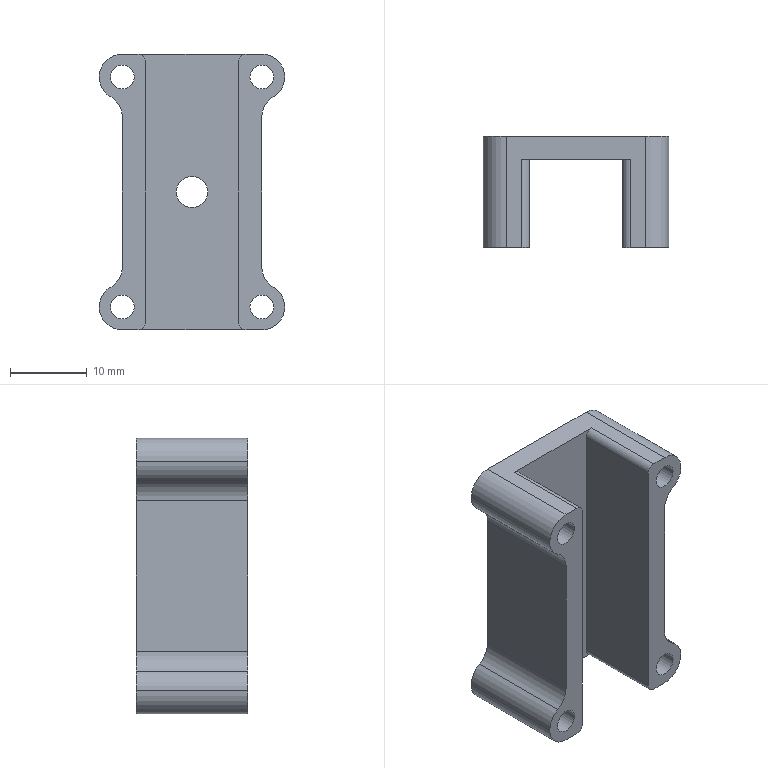Part | SolidWorks | features Fillet 2, ICE 2, Extrusion 1 | 1 solid | 34 faces | box 24.2 x 14.5 x 36 mm | volume 4824 mm3 | cylinder 24 | plane 10 | commonest cylinder face diameters 6 x10 3.1 x8 2 x4 4.1 x2
STEP:
#1=CARTESIAN_POINT('',(2.05,6.,18.));
#2=VERTEX_POINT('',#1);
#3=CARTESIAN_POINT('',(-2.05,6.,18.));
#4=VERTEX_POINT('',#3);
#5=CARTESIAN_POINT('',(0.,6.,18.));
#6=DIRECTION('',(0.,1.,0.));
#7=DIRECTION('',(0.,0.,1.));
#8=AXIS2_PLACEMENT_3D('',#5,#6,#7);
#9=CIRCLE('',#8,2.05);
#10=EDGE_CURVE('',#2,#4,#9,.T.);
#11=ORIENTED_EDGE('',*,*,#10,.F.);
#12=CARTESIAN_POINT('',(2.05,9.,18.));
#13=VERTEX_POINT('',#12);
#14=CARTESIAN_POINT('',(2.05,-5.5,18.));
#15=DIRECTION('',(0.,1.,0.));
#16=VECTOR('',#15,1000.);
#17=LINE('',#14,#16);
#18=EDGE_CURVE('',#2,#13,#17,.T.);
#19=ORIENTED_EDGE('',*,*,#18,.T.);
#20=CARTESIAN_POINT('',(-2.05,9.,18.));
#21=VERTEX_POINT('',#20);
#22=CARTESIAN_POINT('',(0.,9.,18.));
#23=DIRECTION('',(0.,1.,0.));
#24=DIRECTION('',(-1.,0.,0.));
#25=AXIS2_PLACEMENT_3D('',#22,#23,#24);
#26=CIRCLE('',#25,2.05);
#27=EDGE_CURVE('',#13,#21,#26,.T.);
#28=ORIENTED_EDGE('',*,*,#27,.T.);
#29=CARTESIAN_POINT('',(-2.05,-5.5,18.));
#30=DIRECTION('',(0.,1.,0.));
#31=VECTOR('',#30,1000.);
#32=LINE('',#29,#31);
#33=EDGE_CURVE('',#4,#21,#32,.T.);
#34=ORIENTED_EDGE('',*,*,#33,.F.);
#35=EDGE_LOOP('',(#11,#19,#28,#34));
#36=FACE_OUTER_BOUND('',#35,.T.);
#37=CARTESIAN_POINT('',(0.,-5.5,18.));
#38=DIRECTION('',(0.,1.,0.));
#39=DIRECTION('',(-1.,0.,0.));
#40=AXIS2_PLACEMENT_3D('',#37,#38,#39);
#41=CYLINDRICAL_SURFACE('',#40,2.05);
#42=ADVANCED_FACE('',(#36),#41,.F.);
#43=CARTESIAN_POINT('',(10.65,-5.5,33.));
#44=VERTEX_POINT('',#43);
#45=CARTESIAN_POINT('',(7.55,-5.5,33.));
#46=VERTEX_POINT('',#45);
#47=CARTESIAN_POINT('',(9.1,-5.5,33.));
#48=DIRECTION('',(0.,1.,0.));
#49=DIRECTION('',(-1.,0.,0.));
#50=AXIS2_PLACEMENT_3D('',#47,#48,#49);
#51=CIRCLE('',#50,1.55);
#52=EDGE_CURVE('',#44,#46,#51,.T.);
#53=ORIENTED_EDGE('',*,*,#52,.F.);
#54=CARTESIAN_POINT('',(10.65,9.,33.));
#55=VERTEX_POINT('',#54);
#56=CARTESIAN_POINT('',(10.65,-5.5,33.));
#57=DIRECTION('',(0.,1.,0.));
#58=VECTOR('',#57,1000.);
#59=LINE('',#56,#58);
#60=EDGE_CURVE('',#44,#55,#59,.T.);
#61=ORIENTED_EDGE('',*,*,#60,.T.);
#62=CARTESIAN_POINT('',(7.55,9.,33.));
#63=VERTEX_POINT('',#62);
#64=CARTESIAN_POINT('',(9.1,9.,33.));
#65=DIRECTION('',(0.,1.,0.));
#66=DIRECTION('',(-1.,0.,0.));
#67=AXIS2_PLACEMENT_3D('',#64,#65,#66);
#68=CIRCLE('',#67,1.55);
#69=EDGE_CURVE('',#55,#63,#68,.T.);
#70=ORIENTED_EDGE('',*,*,#69,.T.);
#71=CARTESIAN_POINT('',(7.55,-5.5,33.));
#72=DIRECTION('',(0.,1.,0.));
#73=VECTOR('',#72,1000.);
#74=LINE('',#71,#73);
#75=EDGE_CURVE('',#46,#63,#74,.T.);
#76=ORIENTED_EDGE('',*,*,#75,.F.);
#77=EDGE_LOOP('',(#53,#61,#70,#76));
#78=FACE_OUTER_BOUND('',#77,.T.);
#79=CARTESIAN_POINT('',(9.1,-5.5,33.));
#80=DIRECTION('',(0.,1.,0.));
#81=DIRECTION('',(-1.,0.,0.));
#82=AXIS2_PLACEMENT_3D('',#79,#80,#81);
#83=CYLINDRICAL_SURFACE('',#82,1.55);
#84=ADVANCED_FACE('',(#78),#83,.F.);
#85=CARTESIAN_POINT('',(10.65,-5.5,3.));
#86=VERTEX_POINT('',#85);
#87=CARTESIAN_POINT('',(7.55,-5.5,3.));
#88=VERTEX_POINT('',#87);
#89=CARTESIAN_POINT('',(9.1,-5.5,3.));
#90=DIRECTION('',(0.,1.,0.));
#91=DIRECTION('',(-1.,0.,0.));
#92=AXIS2_PLACEMENT_3D('',#89,#90,#91);
#93=CIRCLE('',#92,1.55);
#94=EDGE_CURVE('',#86,#88,#93,.T.);
#95=ORIENTED_EDGE('',*,*,#94,.F.);
#96=CARTESIAN_POINT('',(10.65,9.,3.));
#97=VERTEX_POINT('',#96);
#98=CARTESIAN_POINT('',(10.65,-5.5,3.));
#99=DIRECTION('',(0.,1.,0.));
#100=VECTOR('',#99,1000.);
#101=LINE('',#98,#100);
#102=EDGE_CURVE('',#86,#97,#101,.T.);
#103=ORIENTED_EDGE('',*,*,#102,.T.);
#104=CARTESIAN_POINT('',(7.55,9.,3.));
#105=VERTEX_POINT('',#104);
#106=CARTESIAN_POINT('',(9.1,9.,3.));
#107=DIRECTION('',(0.,1.,0.));
#108=DIRECTION('',(-1.,0.,0.));
#109=AXIS2_PLACEMENT_3D('',#106,#107,#108);
#110=CIRCLE('',#109,1.55);
#111=EDGE_CURVE('',#97,#105,#110,.T.);
#112=ORIENTED_EDGE('',*,*,#111,.T.);
#113=CARTESIAN_POINT('',(7.55,-5.5,3.));
#114=DIRECTION('',(0.,1.,0.));
#115=VECTOR('',#114,1000.);
#116=LINE('',#113,#115);
#117=EDGE_CURVE('',#88,#105,#116,.T.);
#118=ORIENTED_EDGE('',*,*,#117,.F.);
#119=EDGE_LOOP('',(#95,#103,#112,#118));
#120=FACE_OUTER_BOUND('',#119,.T.);
#121=CARTESIAN_POINT('',(9.1,-5.5,3.));
#122=DIRECTION('',(0.,1.,0.));
#123=DIRECTION('',(-1.,0.,0.));
#124=AXIS2_PLACEMENT_3D('',#121,#122,#123);
#125=CYLINDRICAL_SURFACE('',#124,1.55);
#126=ADVANCED_FACE('',(#120),#125,.F.);
#127=CARTESIAN_POINT('',(-7.55,-5.5,3.));
#128=VERTEX_POINT('',#127);
#129=CARTESIAN_POINT('',(-10.65,-5.5,3.));
#130=VERTEX_POINT('',#129);
#131=CARTESIAN_POINT('',(-9.1,-5.5,3.));
#132=DIRECTION('',(0.,1.,0.));
#133=DIRECTION('',(-1.,0.,0.));
#134=AXIS2_PLACEMENT_3D('',#131,#132,#133);
#135=CIRCLE('',#134,1.55);
#136=EDGE_CURVE('',#128,#130,#135,.T.);
#137=ORIENTED_EDGE('',*,*,#136,.F.);
#138=CARTESIAN_POINT('',(-7.55,9.,3.));
#139=VERTEX_POINT('',#138);
#140=CARTESIAN_POINT('',(-7.55,-5.5,3.));
#141=DIRECTION('',(0.,1.,0.));
#142=VECTOR('',#141,1000.);
#143=LINE('',#140,#142);
#144=EDGE_CURVE('',#128,#139,#143,.T.);
#145=ORIENTED_EDGE('',*,*,#144,.T.);
#146=CARTESIAN_POINT('',(-10.65,9.,3.));
#147=VERTEX_POINT('',#146);
#148=CARTESIAN_POINT('',(-9.1,9.,3.));
#149=DIRECTION('',(0.,1.,0.));
#150=DIRECTION('',(-1.,0.,0.));
#151=AXIS2_PLACEMENT_3D('',#148,#149,#150);
#152=CIRCLE('',#151,1.55);
#153=EDGE_CURVE('',#139,#147,#152,.T.);
#154=ORIENTED_EDGE('',*,*,#153,.T.);
#155=CARTESIAN_POINT('',(-10.65,-5.5,3.));
#156=DIRECTION('',(0.,1.,0.));
#157=VECTOR('',#156,1000.);
#158=LINE('',#155,#157);
#159=EDGE_CURVE('',#130,#147,#158,.T.);
#160=ORIENTED_EDGE('',*,*,#159,.F.);
#161=EDGE_LOOP('',(#137,#145,#154,#160));
#162=FACE_OUTER_BOUND('',#161,.T.);
#163=CARTESIAN_POINT('',(-9.1,-5.5,3.));
#164=DIRECTION('',(0.,1.,0.));
#165=DIRECTION('',(-1.,0.,0.));
#166=AXIS2_PLACEMENT_3D('',#163,#164,#165);
#167=CYLINDRICAL_SURFACE('',#166,1.55);
#168=ADVANCED_FACE('',(#162),#167,.F.);
#169=CARTESIAN_POINT('',(-7.55,-5.5,33.));
#170=VERTEX_POINT('',#169);
#171=CARTESIAN_POINT('',(-10.65,-5.5,33.));
#172=VERTEX_POINT('',#171);
#173=CARTESIAN_POINT('',(-9.1,-5.5,33.));
#174=DIRECTION('',(0.,1.,0.));
#175=DIRECTION('',(-1.,0.,0.));
#176=AXIS2_PLACEMENT_3D('',#173,#174,#175);
#177=CIRCLE('',#176,1.55);
#178=EDGE_CURVE('',#170,#172,#177,.T.);
#179=ORIENTED_EDGE('',*,*,#178,.F.);
#180=CARTESIAN_POINT('',(-7.55,9.,33.));
#181=VERTEX_POINT('',#180);
#182=CARTESIAN_POINT('',(-7.55,-5.5,33.));
#183=DIRECTION('',(0.,1.,0.));
#184=VECTOR('',#183,1000.);
#185=LINE('',#182,#184);
#186=EDGE_CURVE('',#170,#181,#185,.T.);
#187=ORIENTED_EDGE('',*,*,#186,.T.);
#188=CARTESIAN_POINT('',(-10.65,9.,33.));
#189=VERTEX_POINT('',#188);
#190=CARTESIAN_POINT('',(-9.1,9.,33.));
#191=DIRECTION('',(0.,1.,0.));
#192=DIRECTION('',(-1.,0.,0.));
#193=AXIS2_PLACEMENT_3D('',#190,#191,#192);
#194=CIRCLE('',#193,1.55);
#195=EDGE_CURVE('',#181,#189,#194,.T.);
#196=ORIENTED_EDGE('',*,*,#195,.T.);
#197=CARTESIAN_POINT('',(-10.65,-5.5,33.));
#198=DIRECTION('',(0.,1.,0.));
#199=VECTOR('',#198,1000.);
#200=LINE('',#197,#199);
#201=EDGE_CURVE('',#172,#189,#200,.T.);
#202=ORIENTED_EDGE('',*,*,#201,.F.);
#203=EDGE_LOOP('',(#179,#187,#196,#202));
#204=FACE_OUTER_BOUND('',#203,.T.);
#205=CARTESIAN_POINT('',(-9.1,-5.5,33.));
#206=DIRECTION('',(0.,1.,0.));
#207=DIRECTION('',(-1.,0.,0.));
#208=AXIS2_PLACEMENT_3D('',#205,#206,#207);
#209=CYLINDRICAL_SURFACE('',#208,1.55);
#210=ADVANCED_FACE('',(#204),#209,.F.);
#211=CARTESIAN_POINT('',(-12.1,-5.5,33.));
#212=VERTEX_POINT('',#211);
#213=CARTESIAN_POINT('',(-10.6,-5.5,30.402));
#214=VERTEX_POINT('',#213);
#215=CARTESIAN_POINT('',(-9.1,-5.5,33.));
#216=DIRECTION('',(0.,-1.,0.));
#217=DIRECTION('',(-1.,0.,0.));
#218=AXIS2_PLACEMENT_3D('',#215,#216,#217);
#219=CIRCLE('',#218,3.);
#220=EDGE_CURVE('',#212,#214,#219,.T.);
#221=ORIENTED_EDGE('',*,*,#220,.F.);
#222=CARTESIAN_POINT('',(-12.1,9.,33.));
#223=VERTEX_POINT('',#222);
#224=CARTESIAN_POINT('',(-12.1,-13.985,33.));
#225=DIRECTION('',(0.,1.,0.));
#226=VECTOR('',#225,1000.);
#227=LINE('',#224,#226);
#228=EDGE_CURVE('',#212,#223,#227,.T.);
#229=ORIENTED_EDGE('',*,*,#228,.T.);
#230=CARTESIAN_POINT('',(-10.6,9.,30.402));
#231=VERTEX_POINT('',#230);
#232=CARTESIAN_POINT('',(-9.1,9.,33.));
#233=DIRECTION('',(0.,1.,0.));
#234=DIRECTION('',(1.,0.,0.));
#235=AXIS2_PLACEMENT_3D('',#232,#233,#234);
#236=CIRCLE('',#235,3.);
#237=EDGE_CURVE('',#231,#223,#236,.T.);
#238=ORIENTED_EDGE('',*,*,#237,.F.);
#239=CARTESIAN_POINT('',(-10.6,-13.985,30.402));
#240=DIRECTION('',(0.,-1.,0.));
#241=VECTOR('',#240,1000.);
#242=LINE('',#239,#241);
#243=EDGE_CURVE('',#231,#214,#242,.T.);
#244=ORIENTED_EDGE('',*,*,#243,.T.);
#245=EDGE_LOOP('',(#221,#229,#238,#244));
#246=FACE_OUTER_BOUND('',#245,.T.);
#247=CARTESIAN_POINT('',(-9.1,-13.985,33.));
#248=DIRECTION('',(0.,1.,0.));
#249=DIRECTION('',(-1.,0.,0.));
#250=AXIS2_PLACEMENT_3D('',#247,#248,#249);
#251=CYLINDRICAL_SURFACE('',#250,3.);
#252=ADVANCED_FACE('',(#246),#251,.T.);
#253=CARTESIAN_POINT('',(-12.1,-5.5,3.));
#254=VERTEX_POINT('',#253);
#255=CARTESIAN_POINT('',(-9.1,-5.5,0.));
#256=VERTEX_POINT('',#255);
#257=CARTESIAN_POINT('',(-9.1,-5.5,3.));
#258=DIRECTION('',(0.,-1.,0.));
#259=DIRECTION('',(-1.,0.,0.));
#260=AXIS2_PLACEMENT_3D('',#257,#258,#259);
#261=CIRCLE('',#260,3.);
#262=EDGE_CURVE('',#254,#256,#261,.T.);
#263=ORIENTED_EDGE('',*,*,#262,.F.);
#264=CARTESIAN_POINT('',(-12.1,9.,3.));
#265=VERTEX_POINT('',#264);
#266=CARTESIAN_POINT('',(-12.1,-13.985,3.));
#267=DIRECTION('',(0.,1.,0.));
#268=VECTOR('',#267,1000.);
#269=LINE('',#266,#268);
#270=EDGE_CURVE('',#254,#265,#269,.T.);
#271=ORIENTED_EDGE('',*,*,#270,.T.);
#272=CARTESIAN_POINT('',(-9.1,9.,0.));
#273=VERTEX_POINT('',#272);
#274=CARTESIAN_POINT('',(-9.1,9.,3.));
#275=DIRECTION('',(0.,1.,0.));
#276=DIRECTION('',(-1.,0.,0.));
#277=AXIS2_PLACEMENT_3D('',#274,#275,#276);
#278=CIRCLE('',#277,3.);
#279=EDGE_CURVE('',#273,#265,#278,.T.);
#280=ORIENTED_EDGE('',*,*,#279,.F.);
#281=CARTESIAN_POINT('',(-9.1,-5.5,0.));
#282=DIRECTION('',(0.,-1.,0.));
#283=VECTOR('',#282,1000.);
#284=LINE('',#281,#283);
#285=EDGE_CURVE('',#273,#256,#284,.T.);
#286=ORIENTED_EDGE('',*,*,#285,.T.);
#287=EDGE_LOOP('',(#263,#271,#280,#286));
#288=FACE_OUTER_BOUND('',#287,.T.);
#289=CARTESIAN_POINT('',(-9.1,-13.985,3.));
#290=DIRECTION('',(0.,1.,0.));
#291=DIRECTION('',(-1.,0.,0.));
#292=AXIS2_PLACEMENT_3D('',#289,#290,#291);
#293=CYLINDRICAL_SURFACE('',#292,3.);
#294=ADVANCED_FACE('',(#288),#293,.T.);
#295=CARTESIAN_POINT('',(-6.1,-5.5,35.));
#296=VERTEX_POINT('',#295);
#297=CARTESIAN_POINT('',(-6.1,-5.5,1.));
#298=VERTEX_POINT('',#297);
#299=CARTESIAN_POINT('',(-6.1,-5.5,36.));
#300=DIRECTION('',(0.,0.,-1.));
#301=VECTOR('',#300,1000.);
#302=LINE('',#299,#301);
#303=EDGE_CURVE('',#296,#298,#302,.T.);
#304=ORIENTED_EDGE('',*,*,#303,.T.);
#305=CARTESIAN_POINT('',(-6.1,6.,1.));
#306=VERTEX_POINT('',#305);
#307=CARTESIAN_POINT('',(-6.1,6.,1.));
#308=DIRECTION('',(0.,1.,0.));
#309=VECTOR('',#308,1000.);
#310=LINE('',#307,#309);
#311=EDGE_CURVE('',#298,#306,#310,.T.);
#312=ORIENTED_EDGE('',*,*,#311,.T.);
#313=CARTESIAN_POINT('',(-6.1,6.,35.));
#314=VERTEX_POINT('',#313);
#315=CARTESIAN_POINT('',(-6.1,6.,36.));
#316=DIRECTION('',(0.,0.,-1.));
#317=VECTOR('',#316,1000.);
#318=LINE('',#315,#317);
#319=EDGE_CURVE('',#314,#306,#318,.T.);
#320=ORIENTED_EDGE('',*,*,#319,.F.);
#321=CARTESIAN_POINT('',(-6.1,6.,35.));
#322=DIRECTION('',(0.,-1.,0.));
#323=VECTOR('',#322,1000.);
#324=LINE('',#321,#323);
#325=EDGE_CURVE('',#314,#296,#324,.T.);
#326=ORIENTED_EDGE('',*,*,#325,.T.);
#327=EDGE_LOOP('',(#304,#312,#320,#326));
#328=FACE_OUTER_BOUND('',#327,.T.);
#329=CARTESIAN_POINT('',(-6.1,6.,36.));
#330=DIRECTION('',(-1.,0.,0.));
#331=DIRECTION('',(0.,-1.,0.));
#332=AXIS2_PLACEMENT_3D('',#329,#330,#331);
#333=PLANE('',#332);
#334=ADVANCED_FACE('',(#328),#333,.F.);
#335=CARTESIAN_POINT('',(0.,6.,18.));
#336=DIRECTION('',(0.,1.,0.));
#337=DIRECTION('',(0.,0.,1.));
#338=AXIS2_PLACEMENT_3D('',#335,#336,#337);
#339=CIRCLE('',#338,2.05);
#340=EDGE_CURVE('',#4,#2,#339,.T.);
#341=ORIENTED_EDGE('',*,*,#340,.T.);
#342=ORIENTED_EDGE('',*,*,#10,.T.);
#343=EDGE_LOOP('',(#341,#342));
#344=FACE_BOUND('',#343,.T.);
#345=CARTESIAN_POINT('',(-7.1,6.,0.));
#346=VERTEX_POINT('',#345);
#347=CARTESIAN_POINT('',(7.1,6.,0.));
#348=VERTEX_POINT('',#347);
#349=CARTESIAN_POINT('',(-6.1,6.,0.));
#350=DIRECTION('',(1.,0.,0.));
#351=VECTOR('',#350,1000.);
#352=LINE('',#349,#351);
#353=EDGE_CURVE('',#346,#348,#352,.T.);
#354=ORIENTED_EDGE('',*,*,#353,.T.);
#355=CARTESIAN_POINT('',(6.1,6.,1.));
#356=VERTEX_POINT('',#355);
#357=CARTESIAN_POINT('',(7.1,6.,1.));
#358=DIRECTION('',(0.,1.,0.));
#359=DIRECTION('',(0.,0.,1.));
#360=AXIS2_PLACEMENT_3D('',#357,#358,#359);
#361=CIRCLE('',#360,1.);
#362=EDGE_CURVE('',#348,#356,#361,.T.);
#363=ORIENTED_EDGE('',*,*,#362,.T.);
#364=CARTESIAN_POINT('',(6.1,6.,35.));
#365=VERTEX_POINT('',#364);
#366=CARTESIAN_POINT('',(6.1,6.,36.));
#367=DIRECTION('',(0.,0.,-1.));
#368=VECTOR('',#367,1000.);
#369=LINE('',#366,#368);
#370=EDGE_CURVE('',#365,#356,#369,.T.);
#371=ORIENTED_EDGE('',*,*,#370,.F.);
#372=CARTESIAN_POINT('',(7.1,6.,36.));
#373=VERTEX_POINT('',#372);
#374=CARTESIAN_POINT('',(7.1,6.,35.));
#375=DIRECTION('',(0.,1.,0.));
#376=DIRECTION('',(0.,0.,1.));
#377=AXIS2_PLACEMENT_3D('',#374,#375,#376);
#378=CIRCLE('',#377,1.);
#379=EDGE_CURVE('',#365,#373,#378,.T.);
#380=ORIENTED_EDGE('',*,*,#379,.T.);
#381=CARTESIAN_POINT('',(-7.1,6.,36.));
#382=VERTEX_POINT('',#381);
#383=CARTESIAN_POINT('',(-6.1,6.,36.));
#384=DIRECTION('',(1.,0.,0.));
#385=VECTOR('',#384,1000.);
#386=LINE('',#383,#385);
#387=EDGE_CURVE('',#382,#373,#386,.T.);
#388=ORIENTED_EDGE('',*,*,#387,.F.);
#389=CARTESIAN_POINT('',(-7.1,6.,35.));
#390=DIRECTION('',(0.,1.,0.));
#391=DIRECTION('',(0.,0.,1.));
#392=AXIS2_PLACEMENT_3D('',#389,#390,#391);
#393=CIRCLE('',#392,1.);
#394=EDGE_CURVE('',#382,#314,#393,.T.);
#395=ORIENTED_EDGE('',*,*,#394,.T.);
#396=ORIENTED_EDGE('',*,*,#319,.T.);
#397=CARTESIAN_POINT('',(-7.1,6.,1.));
#398=DIRECTION('',(0.,1.,0.));
#399=DIRECTION('',(0.,0.,1.));
#400=AXIS2_PLACEMENT_3D('',#397,#398,#399);
#401=CIRCLE('',#400,1.);
#402=EDGE_CURVE('',#306,#346,#401,.T.);
#403=ORIENTED_EDGE('',*,*,#402,.T.);
#404=EDGE_LOOP('',(#354,#363,#371,#380,#388,#395,#396,#403));
#405=FACE_OUTER_BOUND('',#404,.T.);
#406=CARTESIAN_POINT('',(-6.1,6.,36.));
#407=DIRECTION('',(0.,1.,0.));
#408=DIRECTION('',(0.,0.,1.));
#409=AXIS2_PLACEMENT_3D('',#406,#407,#408);
#410=PLANE('',#409);
#411=ADVANCED_FACE('',(#344,#405),#410,.F.);
#412=ORIENTED_EDGE('',*,*,#370,.T.);
#413=CARTESIAN_POINT('',(6.1,-5.5,1.));
#414=VERTEX_POINT('',#413);
#415=CARTESIAN_POINT('',(6.1,-5.5,1.));
#416=DIRECTION('',(0.,-1.,0.));
#417=VECTOR('',#416,1000.);
#418=LINE('',#415,#417);
#419=EDGE_CURVE('',#356,#414,#418,.T.);
#420=ORIENTED_EDGE('',*,*,#419,.T.);
#421=CARTESIAN_POINT('',(6.1,-5.5,35.));
#422=VERTEX_POINT('',#421);
#423=CARTESIAN_POINT('',(6.1,-5.5,36.));
#424=DIRECTION('',(0.,0.,-1.));
#425=VECTOR('',#424,1000.);
#426=LINE('',#423,#425);
#427=EDGE_CURVE('',#422,#414,#426,.T.);
#428=ORIENTED_EDGE('',*,*,#427,.F.);
#429=CARTESIAN_POINT('',(6.1,-5.5,35.));
#430=DIRECTION('',(0.,1.,0.));
#431=VECTOR('',#430,1000.);
#432=LINE('',#429,#431);
#433=EDGE_CURVE('',#422,#365,#432,.T.);
#434=ORIENTED_EDGE('',*,*,#433,.T.);
#435=EDGE_LOOP('',(#412,#420,#428,#434));
#436=FACE_OUTER_BOUND('',#435,.T.);
#437=CARTESIAN_POINT('',(6.1,-5.5,36.));
#438=DIRECTION('',(1.,0.,0.));
#439=DIRECTION('',(0.,1.,0.));
#440=AXIS2_PLACEMENT_3D('',#437,#438,#439);
#441=PLANE('',#440);
#442=ADVANCED_FACE('',(#436),#441,.F.);
#443=CARTESIAN_POINT('',(9.1,-5.5,33.));
#444=DIRECTION('',(0.,1.,0.));
#445=DIRECTION('',(-1.,0.,0.));
#446=AXIS2_PLACEMENT_3D('',#443,#444,#445);
#447=CIRCLE('',#446,1.55);
#448=EDGE_CURVE('',#46,#44,#447,.T.);
#449=ORIENTED_EDGE('',*,*,#448,.T.);
#450=ORIENTED_EDGE('',*,*,#52,.T.);
#451=EDGE_LOOP('',(#449,#450));
#452=FACE_BOUND('',#451,.T.);
#453=CARTESIAN_POINT('',(9.1,-5.5,3.));
#454=DIRECTION('',(0.,1.,0.));
#455=DIRECTION('',(-1.,0.,0.));
#456=AXIS2_PLACEMENT_3D('',#453,#454,#455);
#457=CIRCLE('',#456,1.55);
#458=EDGE_CURVE('',#88,#86,#457,.T.);
#459=ORIENTED_EDGE('',*,*,#458,.T.);
#460=ORIENTED_EDGE('',*,*,#94,.T.);
#461=EDGE_LOOP('',(#459,#460));
#462=FACE_BOUND('',#461,.T.);
#463=ORIENTED_EDGE('',*,*,#427,.T.);
#464=CARTESIAN_POINT('',(7.1,-5.5,0.));
#465=VERTEX_POINT('',#464);
#466=CARTESIAN_POINT('',(7.1,-5.5,1.));
#467=DIRECTION('',(0.,-1.,0.));
#468=DIRECTION('',(0.,0.,1.));
#469=AXIS2_PLACEMENT_3D('',#466,#467,#468);
#470=CIRCLE('',#469,1.);
#471=EDGE_CURVE('',#414,#465,#470,.T.);
#472=ORIENTED_EDGE('',*,*,#471,.T.);
#473=CARTESIAN_POINT('',(9.1,-5.5,0.));
#474=VERTEX_POINT('',#473);
#475=CARTESIAN_POINT('',(9.1,-5.5,0.));
#476=DIRECTION('',(1.,0.,0.));
#477=VECTOR('',#476,1000.);
#478=LINE('',#475,#477);
#479=EDGE_CURVE('',#465,#474,#478,.T.);
#480=ORIENTED_EDGE('',*,*,#479,.T.);
#481=CARTESIAN_POINT('',(10.6,-5.5,5.598));
#482=VERTEX_POINT('',#481);
#483=CARTESIAN_POINT('',(9.1,-5.5,3.));
#484=DIRECTION('',(0.,-1.,0.));
#485=DIRECTION('',(-1.,0.,0.));
#486=AXIS2_PLACEMENT_3D('',#483,#484,#485);
#487=CIRCLE('',#486,3.);
#488=EDGE_CURVE('',#474,#482,#487,.T.);
#489=ORIENTED_EDGE('',*,*,#488,.T.);
#490=CARTESIAN_POINT('',(9.1,-5.5,8.196));
#491=VERTEX_POINT('',#490);
#492=CARTESIAN_POINT('',(12.1,-5.5,8.196));
#493=DIRECTION('',(0.,1.,0.));
#494=DIRECTION('',(0.,0.,1.));
#495=AXIS2_PLACEMENT_3D('',#492,#493,#494);
#496=CIRCLE('',#495,3.);
#497=EDGE_CURVE('',#482,#491,#496,.T.);
#498=ORIENTED_EDGE('',*,*,#497,.T.);
#499=CARTESIAN_POINT('',(9.1,-5.5,27.804));
#500=VERTEX_POINT('',#499);
#501=CARTESIAN_POINT('',(9.1,-5.5,36.));
#502=DIRECTION('',(0.,0.,-1.));
#503=VECTOR('',#502,1000.);
#504=LINE('',#501,#503);
#505=EDGE_CURVE('',#500,#491,#504,.T.);
#506=ORIENTED_EDGE('',*,*,#505,.F.);
#507=CARTESIAN_POINT('',(10.6,-5.5,30.402));
#508=VERTEX_POINT('',#507);
#509=CARTESIAN_POINT('',(12.1,-5.5,27.804));
#510=DIRECTION('',(0.,1.,0.));
#511=DIRECTION('',(0.,0.,1.));
#512=AXIS2_PLACEMENT_3D('',#509,#510,#511);
#513=CIRCLE('',#512,3.);
#514=EDGE_CURVE('',#500,#508,#513,.T.);
#515=ORIENTED_EDGE('',*,*,#514,.T.);
#516=CARTESIAN_POINT('',(9.1,-5.5,36.));
#517=VERTEX_POINT('',#516);
#518=CARTESIAN_POINT('',(9.1,-5.5,33.));
#519=DIRECTION('',(0.,-1.,0.));
#520=DIRECTION('',(-1.,0.,0.));
#521=AXIS2_PLACEMENT_3D('',#518,#519,#520);
#522=CIRCLE('',#521,3.);
#523=EDGE_CURVE('',#508,#517,#522,.T.);
#524=ORIENTED_EDGE('',*,*,#523,.T.);
#525=CARTESIAN_POINT('',(7.1,-5.5,36.));
#526=VERTEX_POINT('',#525);
#527=CARTESIAN_POINT('',(9.1,-5.5,36.));
#528=DIRECTION('',(1.,0.,0.));
#529=VECTOR('',#528,1000.);
#530=LINE('',#527,#529);
#531=EDGE_CURVE('',#526,#517,#530,.T.);
#532=ORIENTED_EDGE('',*,*,#531,.F.);
#533=CARTESIAN_POINT('',(7.1,-5.5,35.));
#534=DIRECTION('',(0.,-1.,0.));
#535=DIRECTION('',(0.,0.,1.));
#536=AXIS2_PLACEMENT_3D('',#533,#534,#535);
#537=CIRCLE('',#536,1.);
#538=EDGE_CURVE('',#526,#422,#537,.T.);
#539=ORIENTED_EDGE('',*,*,#538,.T.);
#540=EDGE_LOOP('',(#463,#472,#480,#489,#498,#506,#515,#524,#532,#539));
#541=FACE_OUTER_BOUND('',#540,.T.);
#542=CARTESIAN_POINT('',(9.1,-5.5,36.));
#543=DIRECTION('',(0.,1.,0.));
#544=DIRECTION('',(0.,0.,1.));
#545=AXIS2_PLACEMENT_3D('',#542,#543,#544);
#546=PLANE('',#545);
#547=ADVANCED_FACE('',(#452,#462,#541),#546,.F.);
#548=ORIENTED_EDGE('',*,*,#505,.T.);
#549=CARTESIAN_POINT('',(9.1,9.,8.196));
#550=VERTEX_POINT('',#549);
#551=CARTESIAN_POINT('',(9.1,9.,8.196));
#552=DIRECTION('',(0.,1.,0.));
#553=VECTOR('',#552,1000.);
#554=LINE('',#551,#553);
#555=EDGE_CURVE('',#491,#550,#554,.T.);
#556=ORIENTED_EDGE('',*,*,#555,.T.);
#557=CARTESIAN_POINT('',(9.1,9.,27.804));
#558=VERTEX_POINT('',#557);
#559=CARTESIAN_POINT('',(9.1,9.,36.));
#560=DIRECTION('',(0.,0.,-1.));
#561=VECTOR('',#560,1000.);
#562=LINE('',#559,#561);
#563=EDGE_CURVE('',#558,#550,#562,.T.);
#564=ORIENTED_EDGE('',*,*,#563,.F.);
#565=CARTESIAN_POINT('',(9.1,9.,27.804));
#566=DIRECTION('',(0.,-1.,0.));
#567=VECTOR('',#566,1000.);
#568=LINE('',#565,#567);
#569=EDGE_CURVE('',#558,#500,#568,.T.);
#570=ORIENTED_EDGE('',*,*,#569,.T.);
#571=EDGE_LOOP('',(#548,#556,#564,#570));
#572=FACE_OUTER_BOUND('',#571,.T.);
#573=CARTESIAN_POINT('',(9.1,9.,36.));
#574=DIRECTION('',(-1.,0.,0.));
#575=DIRECTION('',(0.,-1.,0.));
#576=AXIS2_PLACEMENT_3D('',#573,#574,#575);
#577=PLANE('',#576);
#578=ADVANCED_FACE('',(#572),#577,.F.);
#579=CARTESIAN_POINT('',(0.,9.,18.));
#580=DIRECTION('',(0.,1.,0.));
#581=DIRECTION('',(-1.,0.,0.));
#582=AXIS2_PLACEMENT_3D('',#579,#580,#581);
#583=CIRCLE('',#582,2.05);
#584=EDGE_CURVE('',#21,#13,#583,.T.);
#585=ORIENTED_EDGE('',*,*,#584,.F.);
#586=ORIENTED_EDGE('',*,*,#27,.F.);
#587=EDGE_LOOP('',(#585,#586));
#588=FACE_BOUND('',#587,.T.);
#589=CARTESIAN_POINT('',(-9.1,9.,3.));
#590=DIRECTION('',(0.,1.,0.));
#591=DIRECTION('',(-1.,0.,0.));
#592=AXIS2_PLACEMENT_3D('',#589,#590,#591);
#593=CIRCLE('',#592,1.55);
#594=EDGE_CURVE('',#147,#139,#593,.T.);
#595=ORIENTED_EDGE('',*,*,#594,.F.);
#596=ORIENTED_EDGE('',*,*,#153,.F.);
#597=EDGE_LOOP('',(#595,#596));
#598=FACE_BOUND('',#597,.T.);
#599=CARTESIAN_POINT('',(9.1,9.,33.));
#600=DIRECTION('',(0.,1.,0.));
#601=DIRECTION('',(-1.,0.,0.));
#602=AXIS2_PLACEMENT_3D('',#599,#600,#601);
#603=CIRCLE('',#602,1.55);
#604=EDGE_CURVE('',#63,#55,#603,.T.);
#605=ORIENTED_EDGE('',*,*,#604,.F.);
#606=ORIENTED_EDGE('',*,*,#69,.F.);
#607=EDGE_LOOP('',(#605,#606));
#608=FACE_BOUND('',#607,.T.);
#609=CARTESIAN_POINT('',(-9.1,9.,33.));
#610=DIRECTION('',(0.,1.,0.));
#611=DIRECTION('',(-1.,0.,0.));
#612=AXIS2_PLACEMENT_3D('',#609,#610,#611);
#613=CIRCLE('',#612,1.55);
#614=EDGE_CURVE('',#189,#181,#613,.T.);
#615=ORIENTED_EDGE('',*,*,#614,.F.);
#616=ORIENTED_EDGE('',*,*,#195,.F.);
#617=EDGE_LOOP('',(#615,#616));
#618=FACE_BOUND('',#617,.T.);
#619=CARTESIAN_POINT('',(9.1,9.,3.));
#620=DIRECTION('',(0.,1.,0.));
#621=DIRECTION('',(-1.,0.,0.));
#622=AXIS2_PLACEMENT_3D('',#619,#620,#621);
#623=CIRCLE('',#622,1.55);
#624=EDGE_CURVE('',#105,#97,#623,.T.);
#625=ORIENTED_EDGE('',*,*,#624,.F.);
#626=ORIENTED_EDGE('',*,*,#111,.F.);
#627=EDGE_LOOP('',(#625,#626));
#628=FACE_BOUND('',#627,.T.);
#629=CARTESIAN_POINT('',(-9.1,9.,27.804));
#630=VERTEX_POINT('',#629);
#631=CARTESIAN_POINT('',(-9.1,9.,8.196));
#632=VERTEX_POINT('',#631);
#633=CARTESIAN_POINT('',(-9.1,9.,36.));
#634=DIRECTION('',(0.,0.,-1.));
#635=VECTOR('',#634,1000.);
#636=LINE('',#633,#635);
#637=EDGE_CURVE('',#630,#632,#636,.T.);
#638=ORIENTED_EDGE('',*,*,#637,.F.);
#639=CARTESIAN_POINT('',(-12.1,9.,27.804));
#640=DIRECTION('',(0.,-1.,0.));
#641=DIRECTION('',(1.,0.,0.));
#642=AXIS2_PLACEMENT_3D('',#639,#640,#641);
#643=CIRCLE('',#642,3.);
#644=EDGE_CURVE('',#630,#231,#643,.T.);
#645=ORIENTED_EDGE('',*,*,#644,.T.);
#646=ORIENTED_EDGE('',*,*,#237,.T.);
#647=CARTESIAN_POINT('',(-9.1,9.,36.));
#648=VERTEX_POINT('',#647);
#649=CARTESIAN_POINT('',(-9.1,9.,33.));
#650=DIRECTION('',(0.,1.,0.));
#651=DIRECTION('',(1.,0.,0.));
#652=AXIS2_PLACEMENT_3D('',#649,#650,#651);
#653=CIRCLE('',#652,3.);
#654=EDGE_CURVE('',#223,#648,#653,.T.);
#655=ORIENTED_EDGE('',*,*,#654,.T.);
#656=CARTESIAN_POINT('',(9.1,9.,36.));
#657=VERTEX_POINT('',#656);
#658=CARTESIAN_POINT('',(-9.1,9.,36.));
#659=DIRECTION('',(-1.,0.,0.));
#660=VECTOR('',#659,1000.);
#661=LINE('',#658,#660);
#662=EDGE_CURVE('',#657,#648,#661,.T.);
#663=ORIENTED_EDGE('',*,*,#662,.F.);
#664=CARTESIAN_POINT('',(10.6,9.,30.402));
#665=VERTEX_POINT('',#664);
#666=CARTESIAN_POINT('',(9.1,9.,33.));
#667=DIRECTION('',(0.,1.,0.));
#668=DIRECTION('',(1.,0.,0.));
#669=AXIS2_PLACEMENT_3D('',#666,#667,#668);
#670=CIRCLE('',#669,3.);
#671=EDGE_CURVE('',#657,#665,#670,.T.);
#672=ORIENTED_EDGE('',*,*,#671,.T.);
#673=CARTESIAN_POINT('',(12.1,9.,27.804));
#674=DIRECTION('',(0.,-1.,0.));
#675=DIRECTION('',(1.,0.,0.));
#676=AXIS2_PLACEMENT_3D('',#673,#674,#675);
#677=CIRCLE('',#676,3.);
#678=EDGE_CURVE('',#665,#558,#677,.T.);
#679=ORIENTED_EDGE('',*,*,#678,.T.);
#680=ORIENTED_EDGE('',*,*,#563,.T.);
#681=CARTESIAN_POINT('',(10.6,9.,5.598));
#682=VERTEX_POINT('',#681);
#683=CARTESIAN_POINT('',(12.1,9.,8.196));
#684=DIRECTION('',(0.,-1.,0.));
#685=DIRECTION('',(1.,0.,0.));
#686=AXIS2_PLACEMENT_3D('',#683,#684,#685);
#687=CIRCLE('',#686,3.);
#688=EDGE_CURVE('',#550,#682,#687,.T.);
#689=ORIENTED_EDGE('',*,*,#688,.T.);
#690=CARTESIAN_POINT('',(9.1,9.,0.));
#691=VERTEX_POINT('',#690);
#692=CARTESIAN_POINT('',(9.1,9.,3.));
#693=DIRECTION('',(0.,1.,0.));
#694=DIRECTION('',(-1.,0.,0.));
#695=AXIS2_PLACEMENT_3D('',#692,#693,#694);
#696=CIRCLE('',#695,3.);
#697=EDGE_CURVE('',#682,#691,#696,.T.);
#698=ORIENTED_EDGE('',*,*,#697,.T.);
#699=CARTESIAN_POINT('',(-9.1,9.,0.));
#700=DIRECTION('',(-1.,0.,0.));
#701=VECTOR('',#700,1000.);
#702=LINE('',#699,#701);
#703=EDGE_CURVE('',#691,#273,#702,.T.);
#704=ORIENTED_EDGE('',*,*,#703,.T.);
#705=ORIENTED_EDGE('',*,*,#279,.T.);
#706=CARTESIAN_POINT('',(-10.6,9.,5.598));
#707=VERTEX_POINT('',#706);
#708=CARTESIAN_POINT('',(-9.1,9.,3.));
#709=DIRECTION('',(0.,1.,0.));
#710=DIRECTION('',(-1.,0.,0.));
#711=AXIS2_PLACEMENT_3D('',#708,#709,#710);
#712=CIRCLE('',#711,3.);
#713=EDGE_CURVE('',#265,#707,#712,.T.);
#714=ORIENTED_EDGE('',*,*,#713,.T.);
#715=CARTESIAN_POINT('',(-12.1,9.,8.196));
#716=DIRECTION('',(0.,-1.,0.));
#717=DIRECTION('',(1.,0.,0.));
#718=AXIS2_PLACEMENT_3D('',#715,#716,#717);
#719=CIRCLE('',#718,3.);
#720=EDGE_CURVE('',#707,#632,#719,.T.);
#721=ORIENTED_EDGE('',*,*,#720,.T.);
#722=EDGE_LOOP('',(#638,#645,#646,#655,#663,#672,#679,#680,#689,#698,#704,#705,#714,#721));
#723=FACE_OUTER_BOUND('',#722,.T.);
#724=CARTESIAN_POINT('',(-9.1,9.,36.));
#725=DIRECTION('',(0.,-1.,0.));
#726=DIRECTION('',(1.,0.,0.));
#727=AXIS2_PLACEMENT_3D('',#724,#725,#726);
#728=PLANE('',#727);
#729=ADVANCED_FACE('',(#588,#598,#608,#618,#628,#723),#728,.F.);
#730=ORIENTED_EDGE('',*,*,#637,.T.);
#731=CARTESIAN_POINT('',(-9.1,-5.5,8.196));
#732=VERTEX_POINT('',#731);
#733=CARTESIAN_POINT('',(-9.1,-5.5,8.196));
#734=DIRECTION('',(0.,-1.,0.));
#735=VECTOR('',#734,1000.);
#736=LINE('',#733,#735);
#737=EDGE_CURVE('',#632,#732,#736,.T.);
#738=ORIENTED_EDGE('',*,*,#737,.T.);
#739=CARTESIAN_POINT('',(-9.1,-5.5,27.804));
#740=VERTEX_POINT('',#739);
#741=CARTESIAN_POINT('',(-9.1,-5.5,36.));
#742=DIRECTION('',(0.,0.,-1.));
#743=VECTOR('',#742,1000.);
#744=LINE('',#741,#743);
#745=EDGE_CURVE('',#740,#732,#744,.T.);
#746=ORIENTED_EDGE('',*,*,#745,.F.);
#747=CARTESIAN_POINT('',(-9.1,-5.5,27.804));
#748=DIRECTION('',(0.,1.,0.));
#749=VECTOR('',#748,1000.);
#750=LINE('',#747,#749);
#751=EDGE_CURVE('',#740,#630,#750,.T.);
#752=ORIENTED_EDGE('',*,*,#751,.T.);
#753=EDGE_LOOP('',(#730,#738,#746,#752));
#754=FACE_OUTER_BOUND('',#753,.T.);
#755=CARTESIAN_POINT('',(-9.1,-5.5,36.));
#756=DIRECTION('',(1.,0.,0.));
#757=DIRECTION('',(0.,0.,-1.));
#758=AXIS2_PLACEMENT_3D('',#755,#756,#757);
#759=PLANE('',#758);
#760=ADVANCED_FACE('',(#754),#759,.F.);
#761=CARTESIAN_POINT('',(-9.1,-5.5,3.));
#762=DIRECTION('',(0.,1.,0.));
#763=DIRECTION('',(-1.,0.,0.));
#764=AXIS2_PLACEMENT_3D('',#761,#762,#763);
#765=CIRCLE('',#764,1.55);
#766=EDGE_CURVE('',#130,#128,#765,.T.);
#767=ORIENTED_EDGE('',*,*,#766,.T.);
#768=ORIENTED_EDGE('',*,*,#136,.T.);
#769=EDGE_LOOP('',(#767,#768));
#770=FACE_BOUND('',#769,.T.);
#771=CARTESIAN_POINT('',(-9.1,-5.5,33.));
#772=DIRECTION('',(0.,1.,0.));
#773=DIRECTION('',(-1.,0.,0.));
#774=AXIS2_PLACEMENT_3D('',#771,#772,#773);
#775=CIRCLE('',#774,1.55);
#776=EDGE_CURVE('',#172,#170,#775,.T.);
#777=ORIENTED_EDGE('',*,*,#776,.T.);
#778=ORIENTED_EDGE('',*,*,#178,.T.);
#779=EDGE_LOOP('',(#777,#778));
#780=FACE_BOUND('',#779,.T.);
#781=CARTESIAN_POINT('',(-7.1,-5.5,0.));
#782=VERTEX_POINT('',#781);
#783=CARTESIAN_POINT('',(-6.1,-5.5,0.));
#784=DIRECTION('',(1.,0.,0.));
#785=VECTOR('',#784,1000.);
#786=LINE('',#783,#785);
#787=EDGE_CURVE('',#256,#782,#786,.T.);
#788=ORIENTED_EDGE('',*,*,#787,.T.);
#789=CARTESIAN_POINT('',(-7.1,-5.5,1.));
#790=DIRECTION('',(0.,-1.,0.));
#791=DIRECTION('',(-1.,0.,0.));
#792=AXIS2_PLACEMENT_3D('',#789,#790,#791);
#793=CIRCLE('',#792,1.);
#794=EDGE_CURVE('',#782,#298,#793,.T.);
#795=ORIENTED_EDGE('',*,*,#794,.T.);
#796=ORIENTED_EDGE('',*,*,#303,.F.);
#797=CARTESIAN_POINT('',(-7.1,-5.5,36.));
#798=VERTEX_POINT('',#797);
#799=CARTESIAN_POINT('',(-7.1,-5.5,35.));
#800=DIRECTION('',(0.,-1.,0.));
#801=DIRECTION('',(-1.,0.,0.));
#802=AXIS2_PLACEMENT_3D('',#799,#800,#801);
#803=CIRCLE('',#802,1.);
#804=EDGE_CURVE('',#296,#798,#803,.T.);
#805=ORIENTED_EDGE('',*,*,#804,.T.);
#806=CARTESIAN_POINT('',(-9.1,-5.5,36.));
#807=VERTEX_POINT('',#806);
#808=CARTESIAN_POINT('',(-6.1,-5.5,36.));
#809=DIRECTION('',(1.,0.,0.));
#810=VECTOR('',#809,1000.);
#811=LINE('',#808,#810);
#812=EDGE_CURVE('',#807,#798,#811,.T.);
#813=ORIENTED_EDGE('',*,*,#812,.F.);
#814=CARTESIAN_POINT('',(-9.1,-5.5,33.));
#815=DIRECTION('',(0.,-1.,0.));
#816=DIRECTION('',(-1.,0.,0.));
#817=AXIS2_PLACEMENT_3D('',#814,#815,#816);
#818=CIRCLE('',#817,3.);
#819=EDGE_CURVE('',#807,#212,#818,.T.);
#820=ORIENTED_EDGE('',*,*,#819,.T.);
#821=ORIENTED_EDGE('',*,*,#220,.T.);
#822=CARTESIAN_POINT('',(-12.1,-5.5,27.804));
#823=DIRECTION('',(0.,1.,0.));
#824=DIRECTION('',(-1.,0.,0.));
#825=AXIS2_PLACEMENT_3D('',#822,#823,#824);
#826=CIRCLE('',#825,3.);
#827=EDGE_CURVE('',#214,#740,#826,.T.);
#828=ORIENTED_EDGE('',*,*,#827,.T.);
#829=ORIENTED_EDGE('',*,*,#745,.T.);
#830=CARTESIAN_POINT('',(-10.6,-5.5,5.598));
#831=VERTEX_POINT('',#830);
#832=CARTESIAN_POINT('',(-12.1,-5.5,8.196));
#833=DIRECTION('',(0.,1.,0.));
#834=DIRECTION('',(-1.,0.,0.));
#835=AXIS2_PLACEMENT_3D('',#832,#833,#834);
#836=CIRCLE('',#835,3.);
#837=EDGE_CURVE('',#732,#831,#836,.T.);
#838=ORIENTED_EDGE('',*,*,#837,.T.);
#839=CARTESIAN_POINT('',(-9.1,-5.5,3.));
#840=DIRECTION('',(0.,-1.,0.));
#841=DIRECTION('',(-1.,0.,0.));
#842=AXIS2_PLACEMENT_3D('',#839,#840,#841);
#843=CIRCLE('',#842,3.);
#844=EDGE_CURVE('',#831,#254,#843,.T.);
#845=ORIENTED_EDGE('',*,*,#844,.T.);
#846=ORIENTED_EDGE('',*,*,#262,.T.);
#847=EDGE_LOOP('',(#788,#795,#796,#805,#813,#820,#821,#828,#829,#838,#845,#846));
#848=FACE_OUTER_BOUND('',#847,.T.);
#849=CARTESIAN_POINT('',(-6.1,-5.5,36.));
#850=DIRECTION('',(0.,1.,0.));
#851=DIRECTION('',(-1.,0.,0.));
#852=AXIS2_PLACEMENT_3D('',#849,#850,#851);
#853=PLANE('',#852);
#854=ADVANCED_FACE('',(#770,#780,#848),#853,.F.);
#855=ORIENTED_EDGE('',*,*,#387,.T.);
#856=CARTESIAN_POINT('',(7.1,0.,36.));
#857=DIRECTION('',(0.,-1.,0.));
#858=VECTOR('',#857,1000.);
#859=LINE('',#856,#858);
#860=EDGE_CURVE('',#373,#526,#859,.T.);
#861=ORIENTED_EDGE('',*,*,#860,.T.);
#862=ORIENTED_EDGE('',*,*,#531,.T.);
#863=CARTESIAN_POINT('',(9.1,9.,36.));
#864=DIRECTION('',(0.,1.,0.));
#865=VECTOR('',#864,1000.);
#866=LINE('',#863,#865);
#867=EDGE_CURVE('',#517,#657,#866,.T.);
#868=ORIENTED_EDGE('',*,*,#867,.T.);
#869=ORIENTED_EDGE('',*,*,#662,.T.);
#870=CARTESIAN_POINT('',(-9.1,-5.5,36.));
#871=DIRECTION('',(0.,-1.,0.));
#872=VECTOR('',#871,1000.);
#873=LINE('',#870,#872);
#874=EDGE_CURVE('',#648,#807,#873,.T.);
#875=ORIENTED_EDGE('',*,*,#874,.T.);
#876=ORIENTED_EDGE('',*,*,#812,.T.);
#877=CARTESIAN_POINT('',(-7.1,0.,36.));
#878=DIRECTION('',(0.,1.,0.));
#879=VECTOR('',#878,1000.);
#880=LINE('',#877,#879);
#881=EDGE_CURVE('',#798,#382,#880,.T.);
#882=ORIENTED_EDGE('',*,*,#881,.T.);
#883=EDGE_LOOP('',(#855,#861,#862,#868,#869,#875,#876,#882));
#884=FACE_OUTER_BOUND('',#883,.T.);
#885=CARTESIAN_POINT('',(0.,0.,36.));
#886=DIRECTION('',(0.,0.,-1.));
#887=DIRECTION('',(-1.,0.,0.));
#888=AXIS2_PLACEMENT_3D('',#885,#886,#887);
#889=PLANE('',#888);
#890=ADVANCED_FACE('',(#884),#889,.F.);
#891=ORIENTED_EDGE('',*,*,#479,.F.);
#892=CARTESIAN_POINT('',(7.1,6.,0.));
#893=DIRECTION('',(0.,1.,0.));
#894=VECTOR('',#893,1000.);
#895=LINE('',#892,#894);
#896=EDGE_CURVE('',#465,#348,#895,.T.);
#897=ORIENTED_EDGE('',*,*,#896,.T.);
#898=ORIENTED_EDGE('',*,*,#353,.F.);
#899=CARTESIAN_POINT('',(-7.1,-5.5,0.));
#900=DIRECTION('',(0.,-1.,0.));
#901=VECTOR('',#900,1000.);
#902=LINE('',#899,#901);
#903=EDGE_CURVE('',#346,#782,#902,.T.);
#904=ORIENTED_EDGE('',*,*,#903,.T.);
#905=ORIENTED_EDGE('',*,*,#787,.F.);
#906=ORIENTED_EDGE('',*,*,#285,.F.);
#907=ORIENTED_EDGE('',*,*,#703,.F.);
#908=CARTESIAN_POINT('',(9.1,9.,0.));
#909=DIRECTION('',(0.,1.,0.));
#910=VECTOR('',#909,1000.);
#911=LINE('',#908,#910);
#912=EDGE_CURVE('',#474,#691,#911,.T.);
#913=ORIENTED_EDGE('',*,*,#912,.F.);
#914=EDGE_LOOP('',(#891,#897,#898,#904,#905,#906,#907,#913));
#915=FACE_OUTER_BOUND('',#914,.T.);
#916=CARTESIAN_POINT('',(0.,0.,0.));
#917=DIRECTION('',(0.,0.,-1.));
#918=DIRECTION('',(-1.,0.,0.));
#919=AXIS2_PLACEMENT_3D('',#916,#917,#918);
#920=PLANE('',#919);
#921=ADVANCED_FACE('',(#915),#920,.T.);
#922=ORIENTED_EDGE('',*,*,#697,.F.);
#923=CARTESIAN_POINT('',(10.6,-13.985,5.598));
#924=DIRECTION('',(0.,-1.,0.));
#925=VECTOR('',#924,1000.);
#926=LINE('',#923,#925);
#927=EDGE_CURVE('',#682,#482,#926,.T.);
#928=ORIENTED_EDGE('',*,*,#927,.T.);
#929=ORIENTED_EDGE('',*,*,#488,.F.);
#930=ORIENTED_EDGE('',*,*,#912,.T.);
#931=EDGE_LOOP('',(#922,#928,#929,#930));
#932=FACE_OUTER_BOUND('',#931,.T.);
#933=CARTESIAN_POINT('',(9.1,-13.985,3.));
#934=DIRECTION('',(0.,1.,0.));
#935=DIRECTION('',(-1.,0.,0.));
#936=AXIS2_PLACEMENT_3D('',#933,#934,#935);
#937=CYLINDRICAL_SURFACE('',#936,3.);
#938=ADVANCED_FACE('',(#932),#937,.T.);
#939=ORIENTED_EDGE('',*,*,#270,.F.);
#940=ORIENTED_EDGE('',*,*,#844,.F.);
#941=CARTESIAN_POINT('',(-10.6,-13.985,5.598));
#942=DIRECTION('',(0.,1.,0.));
#943=VECTOR('',#942,1000.);
#944=LINE('',#941,#943);
#945=EDGE_CURVE('',#831,#707,#944,.T.);
#946=ORIENTED_EDGE('',*,*,#945,.T.);
#947=ORIENTED_EDGE('',*,*,#713,.F.);
#948=EDGE_LOOP('',(#939,#940,#946,#947));
#949=FACE_OUTER_BOUND('',#948,.T.);
#950=CARTESIAN_POINT('',(-9.1,-13.985,3.));
#951=DIRECTION('',(0.,1.,0.));
#952=DIRECTION('',(-1.,0.,0.));
#953=AXIS2_PLACEMENT_3D('',#950,#951,#952);
#954=CYLINDRICAL_SURFACE('',#953,3.);
#955=ADVANCED_FACE('',(#949),#954,.T.);
#956=ORIENTED_EDGE('',*,*,#523,.F.);
#957=CARTESIAN_POINT('',(10.6,-13.985,30.402));
#958=DIRECTION('',(0.,1.,0.));
#959=VECTOR('',#958,1000.);
#960=LINE('',#957,#959);
#961=EDGE_CURVE('',#508,#665,#960,.T.);
#962=ORIENTED_EDGE('',*,*,#961,.T.);
#963=ORIENTED_EDGE('',*,*,#671,.F.);
#964=ORIENTED_EDGE('',*,*,#867,.F.);
#965=EDGE_LOOP('',(#956,#962,#963,#964));
#966=FACE_OUTER_BOUND('',#965,.T.);
#967=CARTESIAN_POINT('',(9.1,-13.985,33.));
#968=DIRECTION('',(0.,1.,0.));
#969=DIRECTION('',(-1.,0.,0.));
#970=AXIS2_PLACEMENT_3D('',#967,#968,#969);
#971=CYLINDRICAL_SURFACE('',#970,3.);
#972=ADVANCED_FACE('',(#966),#971,.T.);
#973=ORIENTED_EDGE('',*,*,#228,.F.);
#974=ORIENTED_EDGE('',*,*,#819,.F.);
#975=ORIENTED_EDGE('',*,*,#874,.F.);
#976=ORIENTED_EDGE('',*,*,#654,.F.);
#977=EDGE_LOOP('',(#973,#974,#975,#976));
#978=FACE_OUTER_BOUND('',#977,.T.);
#979=CARTESIAN_POINT('',(-9.1,-13.985,33.));
#980=DIRECTION('',(0.,1.,0.));
#981=DIRECTION('',(-1.,0.,0.));
#982=AXIS2_PLACEMENT_3D('',#979,#980,#981);
#983=CYLINDRICAL_SURFACE('',#982,3.);
#984=ADVANCED_FACE('',(#978),#983,.T.);
#985=ORIENTED_EDGE('',*,*,#186,.F.);
#986=ORIENTED_EDGE('',*,*,#776,.F.);
#987=ORIENTED_EDGE('',*,*,#201,.T.);
#988=ORIENTED_EDGE('',*,*,#614,.T.);
#989=EDGE_LOOP('',(#985,#986,#987,#988));
#990=FACE_OUTER_BOUND('',#989,.T.);
#991=CARTESIAN_POINT('',(-9.1,-5.5,33.));
#992=DIRECTION('',(0.,1.,0.));
#993=DIRECTION('',(-1.,0.,0.));
#994=AXIS2_PLACEMENT_3D('',#991,#992,#993);
#995=CYLINDRICAL_SURFACE('',#994,1.55);
#996=ADVANCED_FACE('',(#990),#995,.F.);
#997=ORIENTED_EDGE('',*,*,#144,.F.);
#998=ORIENTED_EDGE('',*,*,#766,.F.);
#999=ORIENTED_EDGE('',*,*,#159,.T.);
#1000=ORIENTED_EDGE('',*,*,#594,.T.);
#1001=EDGE_LOOP('',(#997,#998,#999,#1000));
#1002=FACE_OUTER_BOUND('',#1001,.T.);
#1003=CARTESIAN_POINT('',(-9.1,-5.5,3.));
#1004=DIRECTION('',(0.,1.,0.));
#1005=DIRECTION('',(-1.,0.,0.));
#1006=AXIS2_PLACEMENT_3D('',#1003,#1004,#1005);
#1007=CYLINDRICAL_SURFACE('',#1006,1.55);
#1008=ADVANCED_FACE('',(#1002),#1007,.F.);
#1009=ORIENTED_EDGE('',*,*,#102,.F.);
#1010=ORIENTED_EDGE('',*,*,#458,.F.);
#1011=ORIENTED_EDGE('',*,*,#117,.T.);
#1012=ORIENTED_EDGE('',*,*,#624,.T.);
#1013=EDGE_LOOP('',(#1009,#1010,#1011,#1012));
#1014=FACE_OUTER_BOUND('',#1013,.T.);
#1015=CARTESIAN_POINT('',(9.1,-5.5,3.));
#1016=DIRECTION('',(0.,1.,0.));
#1017=DIRECTION('',(-1.,0.,0.));
#1018=AXIS2_PLACEMENT_3D('',#1015,#1016,#1017);
#1019=CYLINDRICAL_SURFACE('',#1018,1.55);
#1020=ADVANCED_FACE('',(#1014),#1019,.F.);
#1021=ORIENTED_EDGE('',*,*,#60,.F.);
#1022=ORIENTED_EDGE('',*,*,#448,.F.);
#1023=ORIENTED_EDGE('',*,*,#75,.T.);
#1024=ORIENTED_EDGE('',*,*,#604,.T.);
#1025=EDGE_LOOP('',(#1021,#1022,#1023,#1024));
#1026=FACE_OUTER_BOUND('',#1025,.T.);
#1027=CARTESIAN_POINT('',(9.1,-5.5,33.));
#1028=DIRECTION('',(0.,1.,0.));
#1029=DIRECTION('',(-1.,0.,0.));
#1030=AXIS2_PLACEMENT_3D('',#1027,#1028,#1029);
#1031=CYLINDRICAL_SURFACE('',#1030,1.55);
#1032=ADVANCED_FACE('',(#1026),#1031,.F.);
#1033=ORIENTED_EDGE('',*,*,#18,.F.);
#1034=ORIENTED_EDGE('',*,*,#340,.F.);
#1035=ORIENTED_EDGE('',*,*,#33,.T.);
#1036=ORIENTED_EDGE('',*,*,#584,.T.);
#1037=EDGE_LOOP('',(#1033,#1034,#1035,#1036));
#1038=FACE_OUTER_BOUND('',#1037,.T.);
#1039=CARTESIAN_POINT('',(0.,-5.5,18.));
#1040=DIRECTION('',(0.,1.,0.));
#1041=DIRECTION('',(-1.,0.,0.));
#1042=AXIS2_PLACEMENT_3D('',#1039,#1040,#1041);
#1043=CYLINDRICAL_SURFACE('',#1042,2.05);
#1044=ADVANCED_FACE('',(#1038),#1043,.F.);
#1045=ORIENTED_EDGE('',*,*,#720,.F.);
#1046=ORIENTED_EDGE('',*,*,#945,.F.);
#1047=ORIENTED_EDGE('',*,*,#837,.F.);
#1048=ORIENTED_EDGE('',*,*,#737,.F.);
#1049=EDGE_LOOP('',(#1045,#1046,#1047,#1048));
#1050=FACE_OUTER_BOUND('',#1049,.T.);
#1051=CARTESIAN_POINT('',(-12.1,-13.985,8.196));
#1052=DIRECTION('',(0.,1.,0.));
#1053=DIRECTION('',(-1.,0.,0.));
#1054=AXIS2_PLACEMENT_3D('',#1051,#1052,#1053);
#1055=CYLINDRICAL_SURFACE('',#1054,3.);
#1056=ADVANCED_FACE('',(#1050),#1055,.F.);
#1057=ORIENTED_EDGE('',*,*,#827,.F.);
#1058=ORIENTED_EDGE('',*,*,#243,.F.);
#1059=ORIENTED_EDGE('',*,*,#644,.F.);
#1060=ORIENTED_EDGE('',*,*,#751,.F.);
#1061=EDGE_LOOP('',(#1057,#1058,#1059,#1060));
#1062=FACE_OUTER_BOUND('',#1061,.T.);
#1063=CARTESIAN_POINT('',(-12.1,-13.985,27.804));
#1064=DIRECTION('',(0.,1.,0.));
#1065=DIRECTION('',(-1.,0.,0.));
#1066=AXIS2_PLACEMENT_3D('',#1063,#1064,#1065);
#1067=CYLINDRICAL_SURFACE('',#1066,3.);
#1068=ADVANCED_FACE('',(#1062),#1067,.F.);
#1069=ORIENTED_EDGE('',*,*,#497,.F.);
#1070=ORIENTED_EDGE('',*,*,#927,.F.);
#1071=ORIENTED_EDGE('',*,*,#688,.F.);
#1072=ORIENTED_EDGE('',*,*,#555,.F.);
#1073=EDGE_LOOP('',(#1069,#1070,#1071,#1072));
#1074=FACE_OUTER_BOUND('',#1073,.T.);
#1075=CARTESIAN_POINT('',(12.1,-13.985,8.196));
#1076=DIRECTION('',(0.,1.,0.));
#1077=DIRECTION('',(-1.,0.,0.));
#1078=AXIS2_PLACEMENT_3D('',#1075,#1076,#1077);
#1079=CYLINDRICAL_SURFACE('',#1078,3.);
#1080=ADVANCED_FACE('',(#1074),#1079,.F.);
#1081=ORIENTED_EDGE('',*,*,#678,.F.);
#1082=ORIENTED_EDGE('',*,*,#961,.F.);
#1083=ORIENTED_EDGE('',*,*,#514,.F.);
#1084=ORIENTED_EDGE('',*,*,#569,.F.);
#1085=EDGE_LOOP('',(#1081,#1082,#1083,#1084));
#1086=FACE_OUTER_BOUND('',#1085,.T.);
#1087=CARTESIAN_POINT('',(12.1,-13.985,27.804));
#1088=DIRECTION('',(0.,1.,0.));
#1089=DIRECTION('',(-1.,0.,0.));
#1090=AXIS2_PLACEMENT_3D('',#1087,#1088,#1089);
#1091=CYLINDRICAL_SURFACE('',#1090,3.);
#1092=ADVANCED_FACE('',(#1086),#1091,.F.);
#1093=ORIENTED_EDGE('',*,*,#362,.F.);
#1094=ORIENTED_EDGE('',*,*,#896,.F.);
#1095=ORIENTED_EDGE('',*,*,#471,.F.);
#1096=ORIENTED_EDGE('',*,*,#419,.F.);
#1097=EDGE_LOOP('',(#1093,#1094,#1095,#1096));
#1098=FACE_OUTER_BOUND('',#1097,.T.);
#1099=CARTESIAN_POINT('',(7.1,-5.5,1.));
#1100=DIRECTION('',(0.,1.,0.));
#1101=DIRECTION('',(-1.,0.,0.));
#1102=AXIS2_PLACEMENT_3D('',#1099,#1100,#1101);
#1103=CYLINDRICAL_SURFACE('',#1102,1.);
#1104=ADVANCED_FACE('',(#1098),#1103,.T.);
#1105=ORIENTED_EDGE('',*,*,#794,.F.);
#1106=ORIENTED_EDGE('',*,*,#903,.F.);
#1107=ORIENTED_EDGE('',*,*,#402,.F.);
#1108=ORIENTED_EDGE('',*,*,#311,.F.);
#1109=EDGE_LOOP('',(#1105,#1106,#1107,#1108));
#1110=FACE_OUTER_BOUND('',#1109,.T.);
#1111=CARTESIAN_POINT('',(-7.1,6.,1.));
#1112=DIRECTION('',(0.,-1.,0.));
#1113=DIRECTION('',(1.,0.,0.));
#1114=AXIS2_PLACEMENT_3D('',#1111,#1112,#1113);
#1115=CYLINDRICAL_SURFACE('',#1114,1.);
#1116=ADVANCED_FACE('',(#1110),#1115,.T.);
#1117=ORIENTED_EDGE('',*,*,#379,.F.);
#1118=ORIENTED_EDGE('',*,*,#433,.F.);
#1119=ORIENTED_EDGE('',*,*,#538,.F.);
#1120=ORIENTED_EDGE('',*,*,#860,.F.);
#1121=EDGE_LOOP('',(#1117,#1118,#1119,#1120));
#1122=FACE_OUTER_BOUND('',#1121,.T.);
#1123=CARTESIAN_POINT('',(7.1,0.,35.));
#1124=DIRECTION('',(0.,-1.,0.));
#1125=DIRECTION('',(1.,0.,0.));
#1126=AXIS2_PLACEMENT_3D('',#1123,#1124,#1125);
#1127=CYLINDRICAL_SURFACE('',#1126,1.);
#1128=ADVANCED_FACE('',(#1122),#1127,.T.);
#1129=ORIENTED_EDGE('',*,*,#804,.F.);
#1130=ORIENTED_EDGE('',*,*,#325,.F.);
#1131=ORIENTED_EDGE('',*,*,#394,.F.);
#1132=ORIENTED_EDGE('',*,*,#881,.F.);
#1133=EDGE_LOOP('',(#1129,#1130,#1131,#1132));
#1134=FACE_OUTER_BOUND('',#1133,.T.);
#1135=CARTESIAN_POINT('',(-7.1,0.,35.));
#1136=DIRECTION('',(0.,1.,0.));
#1137=DIRECTION('',(-1.,0.,0.));
#1138=AXIS2_PLACEMENT_3D('',#1135,#1136,#1137);
#1139=CYLINDRICAL_SURFACE('',#1138,1.);
#1140=ADVANCED_FACE('',(#1134),#1139,.T.);
#1141=CLOSED_SHELL('',(#42,#84,#126,#168,#210,#252,#294,#334,#411,#442,#547,#578,#729,#760,#854,#890,#921,#938,#955,#972,#984,#996,#1008,#1020,#1032,#1044,#1056,#1068,#1080,#1092,#1104,#1116,#1128,#1140));
#1142=MANIFOLD_SOLID_BREP('',#1141);
#1143=CARTESIAN_POINT('',(0.,0.,0.));
#1144=DIRECTION('',(0.,0.,1.));
#1145=DIRECTION('',(1.,0.,0.));
#1146=AXIS2_PLACEMENT_3D('',#1143,#1144,#1145);
#1147=(LENGTH_UNIT()NAMED_UNIT(*)SI_UNIT(.MILLI.,.METRE.));
#1148=UNCERTAINTY_MEASURE_WITH_UNIT(LENGTH_MEASURE(0.00001),#1147,'','');
#1149=(NAMED_UNIT(*)PLANE_ANGLE_UNIT()SI_UNIT($,.RADIAN.));
#1150=(NAMED_UNIT(*)SI_UNIT($,.STERADIAN.)SOLID_ANGLE_UNIT());
#1151=(GEOMETRIC_REPRESENTATION_CONTEXT(3)GLOBAL_UNCERTAINTY_ASSIGNED_CONTEXT((#1148))GLOBAL_UNIT_ASSIGNED_CONTEXT((#1147,#1149,#1150))REPRESENTATION_CONTEXT('',''));
#1152=ADVANCED_BREP_SHAPE_REPRESENTATION('',(#1142,#1146),#1151);